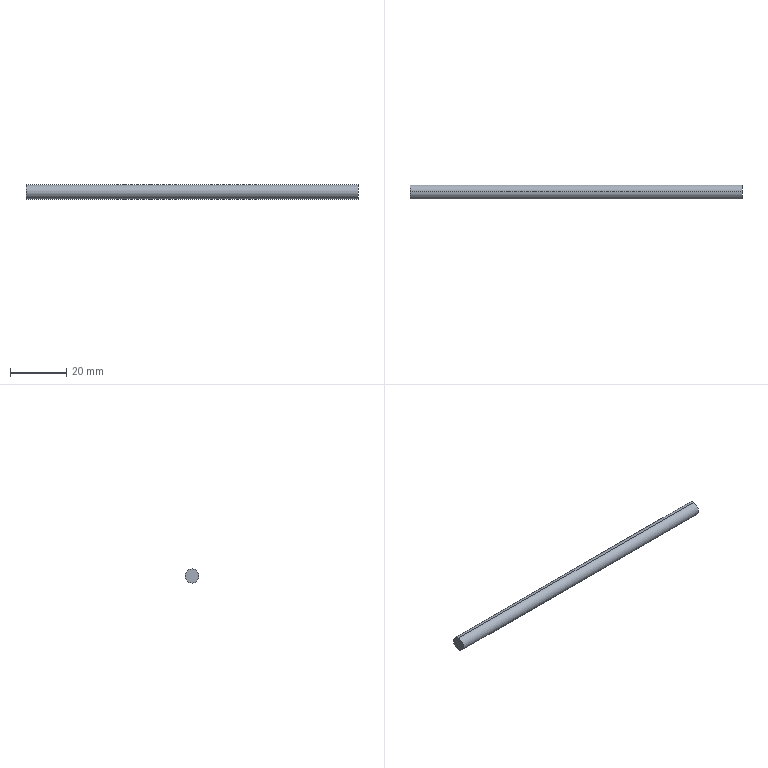Part | SolidWorks | features Extrusion 1 | 1 solid | 4 faces | box 118 x 5 x 5 mm | volume 2317 mm3 | cylinder 2 | plane 2 | commonest cylinder face diameters 5 x2
STEP:
#1=CARTESIAN_POINT('',(118.,0.,-2.5));
#2=VERTEX_POINT('',#1);
#3=CARTESIAN_POINT('',(118.,0.,2.5));
#4=VERTEX_POINT('',#3);
#5=CARTESIAN_POINT('',(118.,0.,0.));
#6=DIRECTION('',(1.,0.,0.));
#7=DIRECTION('',(0.,0.,-1.));
#8=AXIS2_PLACEMENT_3D('',#5,#6,#7);
#9=CIRCLE('',#8,2.5);
#10=EDGE_CURVE('',#2,#4,#9,.T.);
#11=ORIENTED_EDGE('',*,*,#10,.F.);
#12=CARTESIAN_POINT('',(0.,0.,-2.5));
#13=VERTEX_POINT('',#12);
#14=CARTESIAN_POINT('',(118.,0.,-2.5));
#15=DIRECTION('',(-1.,0.,0.));
#16=VECTOR('',#15,1000.);
#17=LINE('',#14,#16);
#18=EDGE_CURVE('',#2,#13,#17,.T.);
#19=ORIENTED_EDGE('',*,*,#18,.T.);
#20=CARTESIAN_POINT('',(0.,0.,2.5));
#21=VERTEX_POINT('',#20);
#22=CARTESIAN_POINT('',(0.,0.,0.));
#23=DIRECTION('',(1.,0.,0.));
#24=DIRECTION('',(0.,0.,-1.));
#25=AXIS2_PLACEMENT_3D('',#22,#23,#24);
#26=CIRCLE('',#25,2.5);
#27=EDGE_CURVE('',#13,#21,#26,.T.);
#28=ORIENTED_EDGE('',*,*,#27,.T.);
#29=CARTESIAN_POINT('',(118.,0.,2.5));
#30=DIRECTION('',(-1.,0.,0.));
#31=VECTOR('',#30,1000.);
#32=LINE('',#29,#31);
#33=EDGE_CURVE('',#4,#21,#32,.T.);
#34=ORIENTED_EDGE('',*,*,#33,.F.);
#35=EDGE_LOOP('',(#11,#19,#28,#34));
#36=FACE_OUTER_BOUND('',#35,.T.);
#37=CARTESIAN_POINT('',(118.,0.,0.));
#38=DIRECTION('',(-1.,0.,0.));
#39=DIRECTION('',(0.,0.,1.));
#40=AXIS2_PLACEMENT_3D('',#37,#38,#39);
#41=CYLINDRICAL_SURFACE('',#40,2.5);
#42=ADVANCED_FACE('',(#36),#41,.T.);
#43=ORIENTED_EDGE('',*,*,#18,.F.);
#44=CARTESIAN_POINT('',(118.,0.,0.));
#45=DIRECTION('',(1.,0.,0.));
#46=DIRECTION('',(0.,0.,-1.));
#47=AXIS2_PLACEMENT_3D('',#44,#45,#46);
#48=CIRCLE('',#47,2.5);
#49=EDGE_CURVE('',#4,#2,#48,.T.);
#50=ORIENTED_EDGE('',*,*,#49,.F.);
#51=ORIENTED_EDGE('',*,*,#33,.T.);
#52=CARTESIAN_POINT('',(0.,0.,0.));
#53=DIRECTION('',(1.,0.,0.));
#54=DIRECTION('',(0.,0.,-1.));
#55=AXIS2_PLACEMENT_3D('',#52,#53,#54);
#56=CIRCLE('',#55,2.5);
#57=EDGE_CURVE('',#21,#13,#56,.T.);
#58=ORIENTED_EDGE('',*,*,#57,.T.);
#59=EDGE_LOOP('',(#43,#50,#51,#58));
#60=FACE_OUTER_BOUND('',#59,.T.);
#61=CARTESIAN_POINT('',(118.,0.,0.));
#62=DIRECTION('',(-1.,0.,0.));
#63=DIRECTION('',(0.,0.,1.));
#64=AXIS2_PLACEMENT_3D('',#61,#62,#63);
#65=CYLINDRICAL_SURFACE('',#64,2.5);
#66=ADVANCED_FACE('',(#60),#65,.T.);
#67=ORIENTED_EDGE('',*,*,#49,.T.);
#68=ORIENTED_EDGE('',*,*,#10,.T.);
#69=EDGE_LOOP('',(#67,#68));
#70=FACE_OUTER_BOUND('',#69,.T.);
#71=CARTESIAN_POINT('',(118.,0.,0.));
#72=DIRECTION('',(1.,0.,0.));
#73=DIRECTION('',(0.,0.,-1.));
#74=AXIS2_PLACEMENT_3D('',#71,#72,#73);
#75=PLANE('',#74);
#76=ADVANCED_FACE('',(#70),#75,.T.);
#77=ORIENTED_EDGE('',*,*,#57,.F.);
#78=ORIENTED_EDGE('',*,*,#27,.F.);
#79=EDGE_LOOP('',(#77,#78));
#80=FACE_OUTER_BOUND('',#79,.T.);
#81=CARTESIAN_POINT('',(0.,0.,0.));
#82=DIRECTION('',(1.,0.,0.));
#83=DIRECTION('',(0.,0.,-1.));
#84=AXIS2_PLACEMENT_3D('',#81,#82,#83);
#85=PLANE('',#84);
#86=ADVANCED_FACE('',(#80),#85,.F.);
#87=CLOSED_SHELL('',(#42,#66,#76,#86));
#88=MANIFOLD_SOLID_BREP('',#87);
#89=CARTESIAN_POINT('',(0.,0.,0.));
#90=DIRECTION('',(0.,0.,1.));
#91=DIRECTION('',(1.,0.,0.));
#92=AXIS2_PLACEMENT_3D('',#89,#90,#91);
#93=(LENGTH_UNIT()NAMED_UNIT(*)SI_UNIT(.MILLI.,.METRE.));
#94=UNCERTAINTY_MEASURE_WITH_UNIT(LENGTH_MEASURE(0.00001),#93,'','');
#95=(NAMED_UNIT(*)PLANE_ANGLE_UNIT()SI_UNIT($,.RADIAN.));
#96=(NAMED_UNIT(*)SI_UNIT($,.STERADIAN.)SOLID_ANGLE_UNIT());
#97=(GEOMETRIC_REPRESENTATION_CONTEXT(3)GLOBAL_UNCERTAINTY_ASSIGNED_CONTEXT((#94))GLOBAL_UNIT_ASSIGNED_CONTEXT((#93,#95,#96))REPRESENTATION_CONTEXT('',''));
#98=ADVANCED_BREP_SHAPE_REPRESENTATION('',(#88,#92),#97);